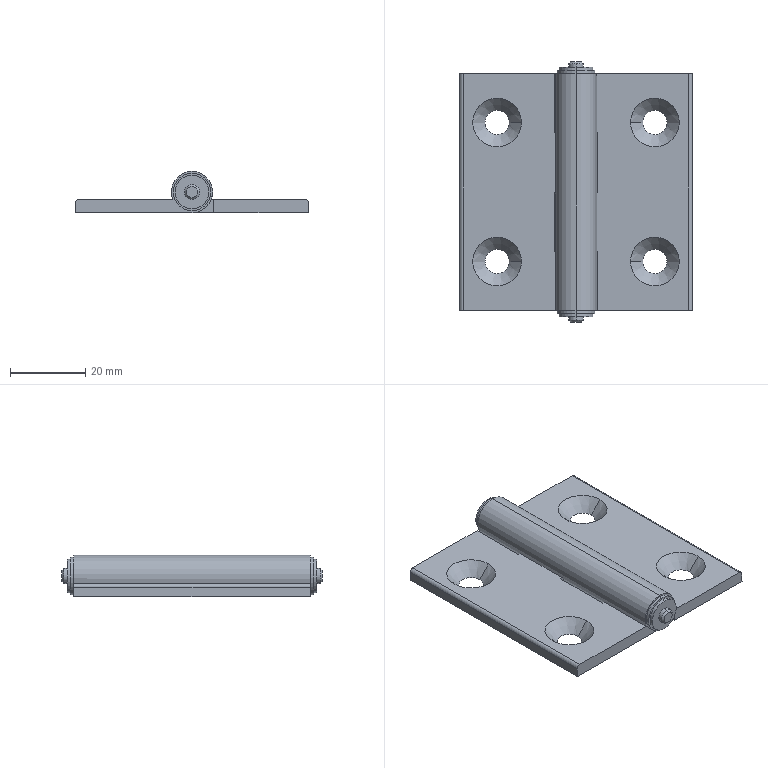Part | SolidWorks | features BaseBody 1 | 1 solid | 54 faces | box 62 x 69.4 x 11 mm | volume 16736 mm3 | plane 26 | cylinder 16 | cone 12 | commonest cylinder face diameters 4 x4 9 x4 10 x4 2 x2 11 x2